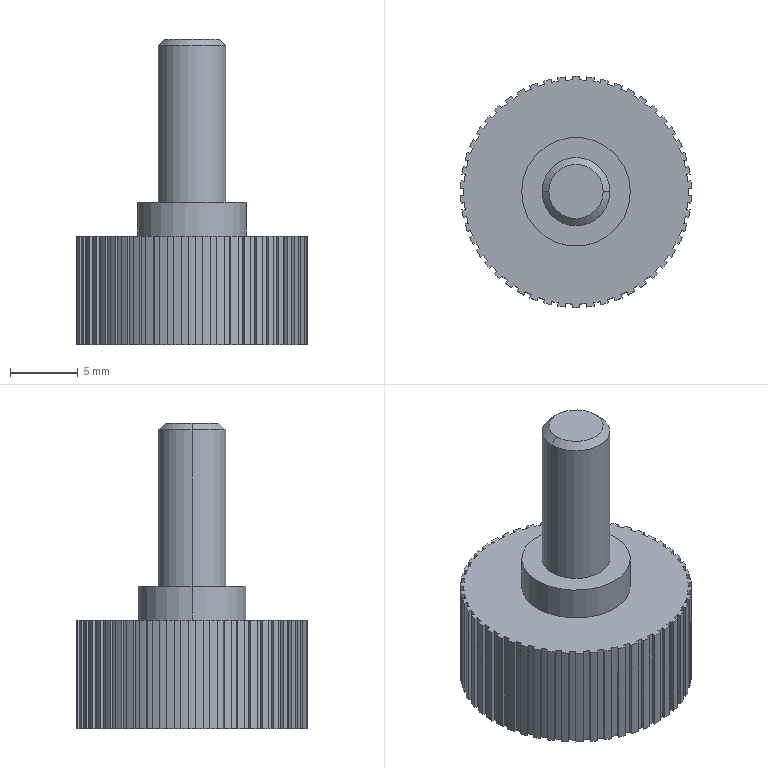Part | SolidWorks | features ICE 3, Chamfer 1, CirPattern 1, Extrusion 1 | 1 solid | 210 faces | box 16.993 x 17 x 22.5 mm | volume 2126 mm3 | plane 154 | cylinder 54 | cone 2 | commonest cylinder face diameters 17 x50 5 x2 8 x2